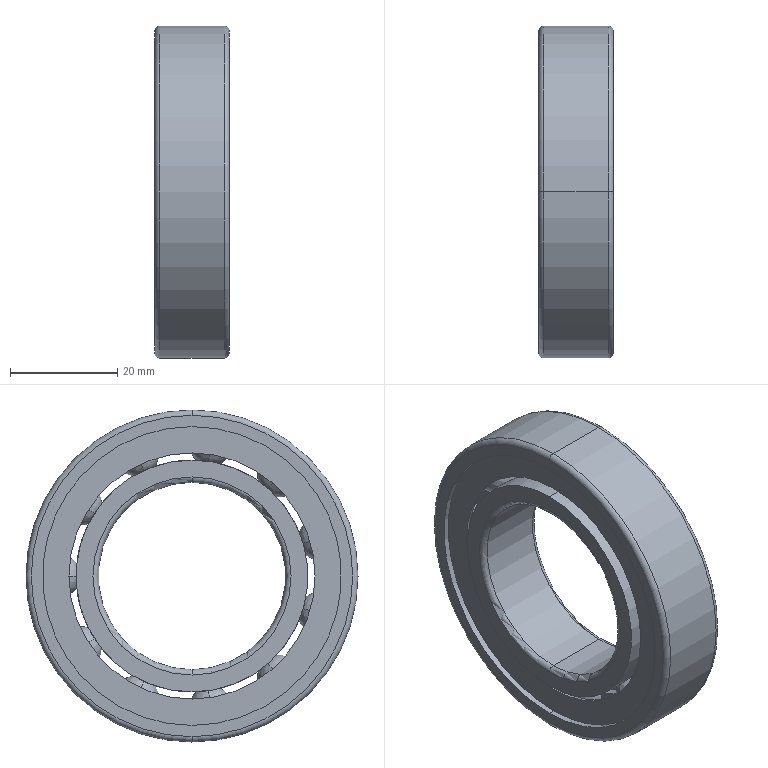Part | STEP file | GB/T276-94 deep groove ball bearing 6007-2Z | 1 solid | 186 faces | box 14 x 62 x 62 mm | volume 18417 mm3 | sphere 88 | torus 44 | plane 30 | cylinder 24 | commonest cylinder face diameters 55.8 x8 43.3 x4 45.94 x4 35 x2 47.35 x2 51.75 x2